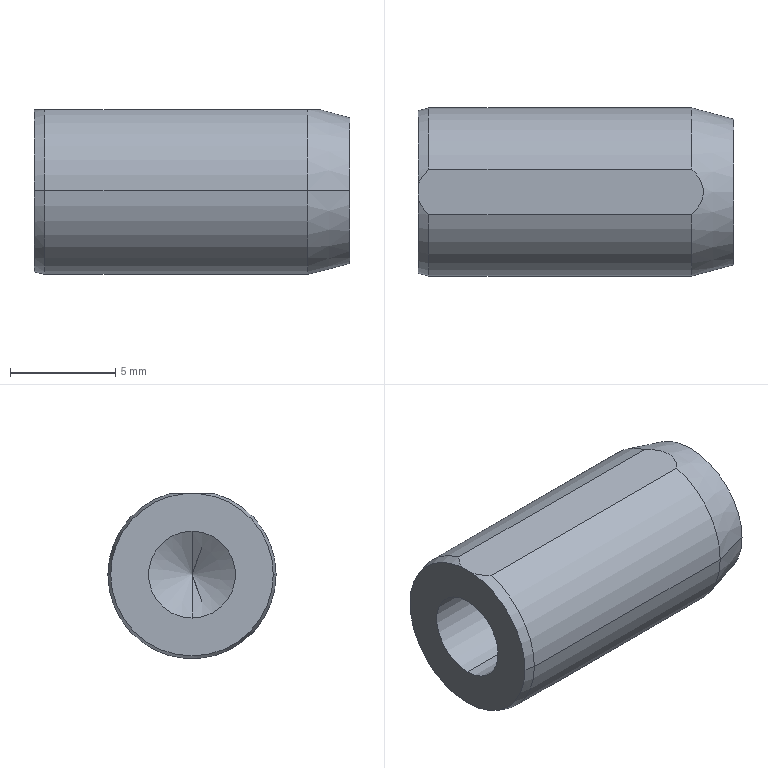Part | STEP file | MSTMS8-15-4 | 1 solid | 15 faces | box 15 x 8 x 7.85 mm | volume 624.527 mm3 | cone 7 | cylinder 5 | plane 3 | commonest cylinder face diameters 8 x3 4.134 x2
STEP:
#1=CARTESIAN_POINT('',(0.,0.,0.));
#2=DIRECTION('',(0.,0.,1.));
#3=DIRECTION('',(1.,0.,0.));
#4=AXIS2_PLACEMENT_3D('',#1,#2,#3);
#5=CARTESIAN_POINT('',(-7.,0.,2.067));
#6=VERTEX_POINT('',#5);
#7=CARTESIAN_POINT('',(-15.,0.,2.067));
#8=VERTEX_POINT('',#7);
#9=CARTESIAN_POINT('',(-15.,0.,2.067));
#10=DIRECTION('',(-1.,0.,0.));
#11=VECTOR('',#10,1.);
#12=LINE('',#9,#11);
#13=CARTESIAN_POINT('',(-15.,0.,0.));
#14=DIRECTION('',(-1.,0.,0.));
#15=DIRECTION('',(0.,0.,1.));
#16=AXIS2_PLACEMENT_3D('',#13,#14,#15);
#17=CYLINDRICAL_SURFACE('',#16,2.067);
#18=CARTESIAN_POINT('',(6.283,0.));
#19=DIRECTION('',(0.,1.));
#20=VECTOR('',#19,1.);
#21=LINE('',#18,#20);
#22=(GEOMETRIC_REPRESENTATION_CONTEXT(2)PARAMETRIC_REPRESENTATION_CONTEXT()REPRESENTATION_CONTEXT('',''));
#23=DEFINITIONAL_REPRESENTATION('',(#21),#22);
#24=PCURVE('',#17,#23);
#25=CARTESIAN_POINT('',(-15.,0.,0.));
#26=DIRECTION('',(-1.,0.,0.));
#27=DIRECTION('',(0.,0.,1.));
#28=AXIS2_PLACEMENT_3D('',#25,#26,#27);
#29=CYLINDRICAL_SURFACE('',#28,2.067);
#30=CARTESIAN_POINT('',(0.,0.));
#31=DIRECTION('',(0.,1.));
#32=VECTOR('',#31,1.);
#33=LINE('',#30,#32);
#34=(GEOMETRIC_REPRESENTATION_CONTEXT(2)PARAMETRIC_REPRESENTATION_CONTEXT()REPRESENTATION_CONTEXT('',''));
#35=DEFINITIONAL_REPRESENTATION('',(#33),#34);
#36=PCURVE('',#29,#35);
#37=SURFACE_CURVE('',#12,(#24,#36),.PCURVE_S1.);
#38=EDGE_CURVE('',#6,#8,#37,.T.);
#39=ORIENTED_EDGE('',*,*,#38,.T.);
#40=CARTESIAN_POINT('',(-15.,0.,-2.067));
#41=VERTEX_POINT('',#40);
#42=CARTESIAN_POINT('',(-15.,0.,0.));
#43=DIRECTION('',(-1.,0.,0.));
#44=DIRECTION('',(0.,0.,1.));
#45=AXIS2_PLACEMENT_3D('',#42,#43,#44);
#46=CIRCLE('',#45,2.067);
#47=CARTESIAN_POINT('',(0.,0.));
#48=DIRECTION('',(1.,0.));
#49=VECTOR('',#48,1.);
#50=LINE('',#47,#49);
#51=(GEOMETRIC_REPRESENTATION_CONTEXT(2)PARAMETRIC_REPRESENTATION_CONTEXT()REPRESENTATION_CONTEXT('',''));
#52=DEFINITIONAL_REPRESENTATION('',(#50),#51);
#53=PCURVE('',#17,#52);
#54=CARTESIAN_POINT('',(-15.,0.,0.));
#55=DIRECTION('',(-1.,0.,0.));
#56=DIRECTION('',(0.,-1.,0.));
#57=AXIS2_PLACEMENT_3D('',#54,#55,#56);
#58=PLANE('',#57);
#59=CARTESIAN_POINT('',(0.,0.));
#60=DIRECTION('',(0.,1.));
#61=AXIS2_PLACEMENT_2D('',#59,#60);
#62=CIRCLE('',#61,2.067);
#63=(GEOMETRIC_REPRESENTATION_CONTEXT(2)PARAMETRIC_REPRESENTATION_CONTEXT()REPRESENTATION_CONTEXT('',''));
#64=DEFINITIONAL_REPRESENTATION('',(#62),#63);
#65=PCURVE('',#58,#64);
#66=SURFACE_CURVE('',#46,(#53,#65),.PCURVE_S1.);
#67=EDGE_CURVE('',#41,#8,#66,.T.);
#68=ORIENTED_EDGE('',*,*,#67,.F.);
#69=CARTESIAN_POINT('',(-7.,0.,-2.067));
#70=VERTEX_POINT('',#69);
#71=CARTESIAN_POINT('',(-15.,0.,-2.067));
#72=DIRECTION('',(-1.,0.,0.));
#73=VECTOR('',#72,1.);
#74=LINE('',#71,#73);
#75=CARTESIAN_POINT('',(3.142,0.));
#76=DIRECTION('',(0.,1.));
#77=VECTOR('',#76,1.);
#78=LINE('',#75,#77);
#79=(GEOMETRIC_REPRESENTATION_CONTEXT(2)PARAMETRIC_REPRESENTATION_CONTEXT()REPRESENTATION_CONTEXT('',''));
#80=DEFINITIONAL_REPRESENTATION('',(#78),#79);
#81=PCURVE('',#17,#80);
#82=CARTESIAN_POINT('',(3.142,0.));
#83=DIRECTION('',(0.,1.));
#84=VECTOR('',#83,1.);
#85=LINE('',#82,#84);
#86=(GEOMETRIC_REPRESENTATION_CONTEXT(2)PARAMETRIC_REPRESENTATION_CONTEXT()REPRESENTATION_CONTEXT('',''));
#87=DEFINITIONAL_REPRESENTATION('',(#85),#86);
#88=PCURVE('',#29,#87);
#89=SURFACE_CURVE('',#74,(#81,#88),.PCURVE_S1.);
#90=EDGE_CURVE('',#70,#41,#89,.T.);
#91=ORIENTED_EDGE('',*,*,#90,.F.);
#92=CARTESIAN_POINT('',(-7.,0.,0.));
#93=DIRECTION('',(-1.,0.,0.));
#94=DIRECTION('',(0.,0.,1.));
#95=AXIS2_PLACEMENT_3D('',#92,#93,#94);
#96=CIRCLE('',#95,2.067);
#97=CARTESIAN_POINT('',(0.,-8.));
#98=DIRECTION('',(1.,0.));
#99=VECTOR('',#98,1.);
#100=LINE('',#97,#99);
#101=(GEOMETRIC_REPRESENTATION_CONTEXT(2)PARAMETRIC_REPRESENTATION_CONTEXT()REPRESENTATION_CONTEXT('',''));
#102=DEFINITIONAL_REPRESENTATION('',(#100),#101);
#103=PCURVE('',#17,#102);
#104=CARTESIAN_POINT('',(-7.,0.,0.));
#105=DIRECTION('',(-1.,0.,0.));
#106=DIRECTION('',(0.,0.,1.));
#107=AXIS2_PLACEMENT_3D('',#104,#105,#106);
#108=CONICAL_SURFACE('',#107,2.067,1.03);
#109=CARTESIAN_POINT('',(0.,0.));
#110=DIRECTION('',(1.,0.));
#111=VECTOR('',#110,1.);
#112=LINE('',#109,#111);
#113=(GEOMETRIC_REPRESENTATION_CONTEXT(2)PARAMETRIC_REPRESENTATION_CONTEXT()REPRESENTATION_CONTEXT('',''));
#114=DEFINITIONAL_REPRESENTATION('',(#112),#113);
#115=PCURVE('',#108,#114);
#116=SURFACE_CURVE('',#96,(#103,#115),.PCURVE_S1.);
#117=EDGE_CURVE('',#70,#6,#116,.T.);
#118=ORIENTED_EDGE('',*,*,#117,.T.);
#119=EDGE_LOOP('',(#39,#68,#91,#118));
#120=FACE_BOUND('',#119,.F.);
#121=ADVANCED_FACE('',(#120),#17,.F.);
#122=ORIENTED_EDGE('',*,*,#117,.F.);
#123=CARTESIAN_POINT('',(-5.758,0.,0.));
#124=VERTEX_POINT('',#123);
#125=CARTESIAN_POINT('',(-7.,0.,-2.067));
#126=DIRECTION('',(-0.515,0.,-0.8572));
#127=VECTOR('',#126,1.);
#128=LINE('',#125,#127);
#129=CARTESIAN_POINT('',(3.142,0.));
#130=DIRECTION('',(0.,1.));
#131=VECTOR('',#130,1.);
#132=LINE('',#129,#131);
#133=(GEOMETRIC_REPRESENTATION_CONTEXT(2)PARAMETRIC_REPRESENTATION_CONTEXT()REPRESENTATION_CONTEXT('',''));
#134=DEFINITIONAL_REPRESENTATION('',(#132),#133);
#135=PCURVE('',#108,#134);
#136=CARTESIAN_POINT('',(-7.,0.,0.));
#137=DIRECTION('',(-1.,0.,0.));
#138=DIRECTION('',(0.,0.,1.));
#139=AXIS2_PLACEMENT_3D('',#136,#137,#138);
#140=CONICAL_SURFACE('',#139,2.067,1.03);
#141=CARTESIAN_POINT('',(3.142,0.));
#142=DIRECTION('',(0.,1.));
#143=VECTOR('',#142,1.);
#144=LINE('',#141,#143);
#145=(GEOMETRIC_REPRESENTATION_CONTEXT(2)PARAMETRIC_REPRESENTATION_CONTEXT()REPRESENTATION_CONTEXT('',''));
#146=DEFINITIONAL_REPRESENTATION('',(#144),#145);
#147=PCURVE('',#140,#146);
#148=SURFACE_CURVE('',#128,(#135,#147),.PCURVE_S1.);
#149=EDGE_CURVE('',#124,#70,#148,.T.);
#150=ORIENTED_EDGE('',*,*,#149,.F.);
#151=CARTESIAN_POINT('',(-7.,0.,2.067));
#152=DIRECTION('',(-0.515,0.,0.8572));
#153=VECTOR('',#152,1.);
#154=LINE('',#151,#153);
#155=CARTESIAN_POINT('',(6.283,0.));
#156=DIRECTION('',(0.,1.));
#157=VECTOR('',#156,1.);
#158=LINE('',#155,#157);
#159=(GEOMETRIC_REPRESENTATION_CONTEXT(2)PARAMETRIC_REPRESENTATION_CONTEXT()REPRESENTATION_CONTEXT('',''));
#160=DEFINITIONAL_REPRESENTATION('',(#158),#159);
#161=PCURVE('',#108,#160);
#162=CARTESIAN_POINT('',(0.,0.));
#163=DIRECTION('',(0.,1.));
#164=VECTOR('',#163,1.);
#165=LINE('',#162,#164);
#166=(GEOMETRIC_REPRESENTATION_CONTEXT(2)PARAMETRIC_REPRESENTATION_CONTEXT()REPRESENTATION_CONTEXT('',''));
#167=DEFINITIONAL_REPRESENTATION('',(#165),#166);
#168=PCURVE('',#140,#167);
#169=SURFACE_CURVE('',#154,(#161,#168),.PCURVE_S1.);
#170=EDGE_CURVE('',#124,#6,#169,.T.);
#171=ORIENTED_EDGE('',*,*,#170,.T.);
#172=EDGE_LOOP('',(#122,#150,#171));
#173=FACE_BOUND('',#172,.F.);
#174=ADVANCED_FACE('',(#173),#108,.F.);
#175=CARTESIAN_POINT('',(0.,3.464,0.));
#176=VERTEX_POINT('',#175);
#177=CARTESIAN_POINT('',(0.,-3.464,0.));
#178=VERTEX_POINT('',#177);
#179=CARTESIAN_POINT('',(0.,0.,0.));
#180=DIRECTION('',(1.,0.,0.));
#181=DIRECTION('',(0.,1.,0.));
#182=AXIS2_PLACEMENT_3D('',#179,#180,#181);
#183=CIRCLE('',#182,3.464);
#184=CARTESIAN_POINT('',(0.,0.,0.));
#185=DIRECTION('',(-1.,0.,0.));
#186=DIRECTION('',(0.,-1.,0.));
#187=AXIS2_PLACEMENT_3D('',#184,#185,#186);
#188=CONICAL_SURFACE('',#187,3.464,0.2618);
#189=CARTESIAN_POINT('',(3.142,0.));
#190=DIRECTION('',(-1.,0.));
#191=VECTOR('',#190,1.);
#192=LINE('',#189,#191);
#193=(GEOMETRIC_REPRESENTATION_CONTEXT(2)PARAMETRIC_REPRESENTATION_CONTEXT()REPRESENTATION_CONTEXT('',''));
#194=DEFINITIONAL_REPRESENTATION('',(#192),#193);
#195=PCURVE('',#188,#194);
#196=CARTESIAN_POINT('',(0.,0.,0.));
#197=DIRECTION('',(1.,0.,0.));
#198=DIRECTION('',(0.,1.,0.));
#199=AXIS2_PLACEMENT_3D('',#196,#197,#198);
#200=PLANE('',#199);
#201=CARTESIAN_POINT('',(0.,0.));
#202=DIRECTION('',(1.,0.));
#203=AXIS2_PLACEMENT_2D('',#201,#202);
#204=CIRCLE('',#203,3.464);
#205=(GEOMETRIC_REPRESENTATION_CONTEXT(2)PARAMETRIC_REPRESENTATION_CONTEXT()REPRESENTATION_CONTEXT('',''));
#206=DEFINITIONAL_REPRESENTATION('',(#204),#205);
#207=PCURVE('',#200,#206);
#208=SURFACE_CURVE('',#183,(#195,#207),.PCURVE_S1.);
#209=EDGE_CURVE('',#176,#178,#208,.T.);
#210=ORIENTED_EDGE('',*,*,#209,.F.);
#211=CARTESIAN_POINT('',(-2.,4.,0.));
#212=VERTEX_POINT('',#211);
#213=CARTESIAN_POINT('',(0.,3.464,0.));
#214=DIRECTION('',(-0.9659,0.2588,0.));
#215=VECTOR('',#214,1.);
#216=LINE('',#213,#215);
#217=CARTESIAN_POINT('',(3.142,0.));
#218=DIRECTION('',(0.,1.));
#219=VECTOR('',#218,1.);
#220=LINE('',#217,#219);
#221=(GEOMETRIC_REPRESENTATION_CONTEXT(2)PARAMETRIC_REPRESENTATION_CONTEXT()REPRESENTATION_CONTEXT('',''));
#222=DEFINITIONAL_REPRESENTATION('',(#220),#221);
#223=PCURVE('',#188,#222);
#224=CARTESIAN_POINT('',(0.,0.,0.));
#225=DIRECTION('',(-1.,0.,0.));
#226=DIRECTION('',(0.,-1.,0.));
#227=AXIS2_PLACEMENT_3D('',#224,#225,#226);
#228=CONICAL_SURFACE('',#227,3.464,0.2618);
#229=CARTESIAN_POINT('',(3.142,0.));
#230=DIRECTION('',(0.,1.));
#231=VECTOR('',#230,1.);
#232=LINE('',#229,#231);
#233=(GEOMETRIC_REPRESENTATION_CONTEXT(2)PARAMETRIC_REPRESENTATION_CONTEXT()REPRESENTATION_CONTEXT('',''));
#234=DEFINITIONAL_REPRESENTATION('',(#232),#233);
#235=PCURVE('',#228,#234);
#236=SURFACE_CURVE('',#216,(#223,#235),.PCURVE_S1.);
#237=EDGE_CURVE('',#176,#212,#236,.T.);
#238=ORIENTED_EDGE('',*,*,#237,.T.);
#239=CARTESIAN_POINT('',(-2.,1.085,3.85));
#240=VERTEX_POINT('',#239);
#241=CARTESIAN_POINT('',(-2.,0.,0.));
#242=DIRECTION('',(1.,0.,0.));
#243=DIRECTION('',(0.,1.,0.));
#244=AXIS2_PLACEMENT_3D('',#241,#242,#243);
#245=CIRCLE('',#244,4.);
#246=CARTESIAN_POINT('',(3.142,2.));
#247=DIRECTION('',(-1.,0.));
#248=VECTOR('',#247,1.);
#249=LINE('',#246,#248);
#250=(GEOMETRIC_REPRESENTATION_CONTEXT(2)PARAMETRIC_REPRESENTATION_CONTEXT()REPRESENTATION_CONTEXT('',''));
#251=DEFINITIONAL_REPRESENTATION('',(#249),#250);
#252=PCURVE('',#188,#251);
#253=CARTESIAN_POINT('',(0.,0.,0.));
#254=DIRECTION('',(1.,0.,0.));
#255=DIRECTION('',(0.,1.,0.));
#256=AXIS2_PLACEMENT_3D('',#253,#254,#255);
#257=CYLINDRICAL_SURFACE('',#256,4.);
#258=CARTESIAN_POINT('',(0.,-2.));
#259=DIRECTION('',(1.,0.));
#260=VECTOR('',#259,1.);
#261=LINE('',#258,#260);
#262=(GEOMETRIC_REPRESENTATION_CONTEXT(2)PARAMETRIC_REPRESENTATION_CONTEXT()REPRESENTATION_CONTEXT('',''));
#263=DEFINITIONAL_REPRESENTATION('',(#261),#262);
#264=PCURVE('',#257,#263);
#265=SURFACE_CURVE('',#245,(#252,#264),.PCURVE_S1.);
#266=EDGE_CURVE('',#212,#240,#265,.T.);
#267=ORIENTED_EDGE('',*,*,#266,.T.);
#268=CARTESIAN_POINT('',(-2.,-1.085,3.85));
#269=VERTEX_POINT('',#268);
#270=CARTESIAN_POINT('',(-2.,-1.085,3.85));
#271=CARTESIAN_POINT('',(-1.853,-0.9403,3.85));
#272=CARTESIAN_POINT('',(-1.716,-0.7784,3.85));
#273=CARTESIAN_POINT('',(-1.508,-0.4159,3.85));
#274=CARTESIAN_POINT('',(-1.44,-0.2099,3.85));
#275=CARTESIAN_POINT('',(-1.44,0.2107,3.85));
#276=CARTESIAN_POINT('',(-1.508,0.4155,3.85));
#277=CARTESIAN_POINT('',(-1.663,0.687,3.85));
#278=CARTESIAN_POINT('',(-1.724,0.7735,3.85));
#279=CARTESIAN_POINT('',(-1.856,0.9358,3.85));
#280=CARTESIAN_POINT('',(-1.926,1.012,3.85));
#281=CARTESIAN_POINT('',(-2.,1.085,3.85));
#282=B_SPLINE_CURVE_WITH_KNOTS('',3,(#270,#271,#272,#273,#274,#275,#276,#277,#278,#279,#280,#281),.UNSPECIFIED.,.F.,.F.,(4,2,2,2,2,4),(0.001238,0.001854,0.00247,0.003086,0.003394,0.003702),.UNSPECIFIED.);
#283=CARTESIAN_POINT('',(1.296,2.));
#284=CARTESIAN_POINT('',(1.302,1.973));
#285=CARTESIAN_POINT('',(1.315,1.921));
#286=CARTESIAN_POINT('',(1.336,1.844));
#287=CARTESIAN_POINT('',(1.358,1.771));
#288=CARTESIAN_POINT('',(1.38,1.703));
#289=CARTESIAN_POINT('',(1.404,1.64));
#290=CARTESIAN_POINT('',(1.429,1.583));
#291=CARTESIAN_POINT('',(1.456,1.534));
#292=CARTESIAN_POINT('',(1.483,1.494));
#293=CARTESIAN_POINT('',(1.512,1.464));
#294=CARTESIAN_POINT('',(1.541,1.445));
#295=CARTESIAN_POINT('',(1.571,1.438));
#296=CARTESIAN_POINT('',(1.601,1.445));
#297=CARTESIAN_POINT('',(1.63,1.464));
#298=CARTESIAN_POINT('',(1.658,1.494));
#299=CARTESIAN_POINT('',(1.686,1.534));
#300=CARTESIAN_POINT('',(1.712,1.583));
#301=CARTESIAN_POINT('',(1.737,1.64));
#302=CARTESIAN_POINT('',(1.761,1.703));
#303=CARTESIAN_POINT('',(1.784,1.772));
#304=CARTESIAN_POINT('',(1.806,1.844));
#305=CARTESIAN_POINT('',(1.826,1.92));
#306=CARTESIAN_POINT('',(1.839,1.973));
#307=CARTESIAN_POINT('',(1.846,2.));
#308=B_SPLINE_CURVE_WITH_KNOTS('',3,(#283,#284,#285,#286,#287,#288,#289,#290,#291,#292,#293,#294,#295,#296,#297,#298,#299,#300,#301,#302,#303,#304,#305,#306,#307),.UNSPECIFIED.,.F.,.F.,(4,1,1,1,1,1,1,1,1,1,1,1,1,1,1,1,1,1,1,1,1,1,4),(0.001238,0.00135,0.001462,0.001574,0.001686,0.001798,0.00191,0.002022,0.002134,0.002246,0.002358,0.00247,0.002582,0.002694,0.002806,0.002918,0.00303,0.003142,0.003254,0.003366,0.003478,0.00359,0.003702),.QUASI_UNIFORM_KNOTS.);
#309=(GEOMETRIC_REPRESENTATION_CONTEXT(2)PARAMETRIC_REPRESENTATION_CONTEXT()REPRESENTATION_CONTEXT('',''));
#310=DEFINITIONAL_REPRESENTATION('',(#308),#309);
#311=PCURVE('',#188,#310);
#312=CARTESIAN_POINT('',(-15.,1.085,3.85));
#313=DIRECTION('',(0.,0.,-1.));
#314=DIRECTION('',(-1.,0.,0.));
#315=AXIS2_PLACEMENT_3D('',#312,#313,#314);
#316=PLANE('',#315);
#317=CARTESIAN_POINT('',(-13.,-2.17));
#318=CARTESIAN_POINT('',(-13.147,-2.025));
#319=CARTESIAN_POINT('',(-13.284,-1.864));
#320=CARTESIAN_POINT('',(-13.492,-1.501));
#321=CARTESIAN_POINT('',(-13.56,-1.295));
#322=CARTESIAN_POINT('',(-13.56,-0.8744));
#323=CARTESIAN_POINT('',(-13.492,-0.6696));
#324=CARTESIAN_POINT('',(-13.337,-0.3981));
#325=CARTESIAN_POINT('',(-13.276,-0.3116));
#326=CARTESIAN_POINT('',(-13.144,-0.1493));
#327=CARTESIAN_POINT('',(-13.074,-0.07297));
#328=CARTESIAN_POINT('',(-13.,0.));
#329=B_SPLINE_CURVE_WITH_KNOTS('',3,(#317,#318,#319,#320,#321,#322,#323,#324,#325,#326,#327,#328),.UNSPECIFIED.,.F.,.F.,(4,2,2,2,2,4),(0.001238,0.001854,0.00247,0.003086,0.003394,0.003702),.UNSPECIFIED.);
#330=(GEOMETRIC_REPRESENTATION_CONTEXT(2)PARAMETRIC_REPRESENTATION_CONTEXT()REPRESENTATION_CONTEXT('',''));
#331=DEFINITIONAL_REPRESENTATION('',(#329),#330);
#332=PCURVE('',#316,#331);
#333=SURFACE_CURVE('',#282,(#311,#332),.PCURVE_S1.);
#334=EDGE_CURVE('',#269,#240,#333,.T.);
#335=ORIENTED_EDGE('',*,*,#334,.F.);
#336=CARTESIAN_POINT('',(-2.,-4.,0.));
#337=VERTEX_POINT('',#336);
#338=CARTESIAN_POINT('',(-2.,0.,0.));
#339=DIRECTION('',(1.,0.,0.));
#340=DIRECTION('',(0.,1.,0.));
#341=AXIS2_PLACEMENT_3D('',#338,#339,#340);
#342=CIRCLE('',#341,4.);
#343=CARTESIAN_POINT('',(3.142,2.));
#344=DIRECTION('',(-1.,0.));
#345=VECTOR('',#344,1.);
#346=LINE('',#343,#345);
#347=(GEOMETRIC_REPRESENTATION_CONTEXT(2)PARAMETRIC_REPRESENTATION_CONTEXT()REPRESENTATION_CONTEXT('',''));
#348=DEFINITIONAL_REPRESENTATION('',(#346),#347);
#349=PCURVE('',#188,#348);
#350=CARTESIAN_POINT('',(0.,0.,0.));
#351=DIRECTION('',(1.,0.,0.));
#352=DIRECTION('',(0.,1.,0.));
#353=AXIS2_PLACEMENT_3D('',#350,#351,#352);
#354=CYLINDRICAL_SURFACE('',#353,4.);
#355=CARTESIAN_POINT('',(0.,-2.));
#356=DIRECTION('',(1.,0.));
#357=VECTOR('',#356,1.);
#358=LINE('',#355,#357);
#359=(GEOMETRIC_REPRESENTATION_CONTEXT(2)PARAMETRIC_REPRESENTATION_CONTEXT()REPRESENTATION_CONTEXT('',''));
#360=DEFINITIONAL_REPRESENTATION('',(#358),#359);
#361=PCURVE('',#354,#360);
#362=SURFACE_CURVE('',#342,(#349,#361),.PCURVE_S1.);
#363=EDGE_CURVE('',#269,#337,#362,.T.);
#364=ORIENTED_EDGE('',*,*,#363,.T.);
#365=CARTESIAN_POINT('',(0.,-3.464,0.));
#366=DIRECTION('',(-0.9659,-0.2588,0.));
#367=VECTOR('',#366,1.);
#368=LINE('',#365,#367);
#369=CARTESIAN_POINT('',(0.,0.));
#370=DIRECTION('',(0.,1.));
#371=VECTOR('',#370,1.);
#372=LINE('',#369,#371);
#373=(GEOMETRIC_REPRESENTATION_CONTEXT(2)PARAMETRIC_REPRESENTATION_CONTEXT()REPRESENTATION_CONTEXT('',''));
#374=DEFINITIONAL_REPRESENTATION('',(#372),#373);
#375=PCURVE('',#188,#374);
#376=CARTESIAN_POINT('',(6.283,0.));
#377=DIRECTION('',(0.,1.));
#378=VECTOR('',#377,1.);
#379=LINE('',#376,#378);
#380=(GEOMETRIC_REPRESENTATION_CONTEXT(2)PARAMETRIC_REPRESENTATION_CONTEXT()REPRESENTATION_CONTEXT('',''));
#381=DEFINITIONAL_REPRESENTATION('',(#379),#380);
#382=PCURVE('',#228,#381);
#383=SURFACE_CURVE('',#368,(#375,#382),.PCURVE_S1.);
#384=EDGE_CURVE('',#178,#337,#383,.T.);
#385=ORIENTED_EDGE('',*,*,#384,.F.);
#386=EDGE_LOOP('',(#210,#238,#267,#335,#364,#385));
#387=FACE_BOUND('',#386,.T.);
#388=ADVANCED_FACE('',(#387),#188,.T.);
#389=CARTESIAN_POINT('',(-14.5,-1.085,3.85));
#390=VERTEX_POINT('',#389);
#391=CARTESIAN_POINT('',(-14.5,-4.,0.));
#392=VERTEX_POINT('',#391);
#393=CARTESIAN_POINT('',(-14.5,0.,0.));
#394=DIRECTION('',(1.,0.,0.));
#395=DIRECTION('',(0.,1.,0.));
#396=AXIS2_PLACEMENT_3D('',#393,#394,#395);
#397=CIRCLE('',#396,4.);
#398=CARTESIAN_POINT('',(0.,-14.5));
#399=DIRECTION('',(1.,0.));
#400=VECTOR('',#399,1.);
#401=LINE('',#398,#400);
#402=(GEOMETRIC_REPRESENTATION_CONTEXT(2)PARAMETRIC_REPRESENTATION_CONTEXT()REPRESENTATION_CONTEXT('',''));
#403=DEFINITIONAL_REPRESENTATION('',(#401),#402);
#404=PCURVE('',#354,#403);
#405=CARTESIAN_POINT('',(-14.5,0.,0.));
#406=DIRECTION('',(1.,0.,0.));
#407=DIRECTION('',(0.,1.,0.));
#408=AXIS2_PLACEMENT_3D('',#405,#406,#407);
#409=CONICAL_SURFACE('',#408,4.,0.2618);
#410=CARTESIAN_POINT('',(0.,0.));
#411=DIRECTION('',(1.,0.));
#412=VECTOR('',#411,1.);
#413=LINE('',#410,#412);
#414=(GEOMETRIC_REPRESENTATION_CONTEXT(2)PARAMETRIC_REPRESENTATION_CONTEXT()REPRESENTATION_CONTEXT('',''));
#415=DEFINITIONAL_REPRESENTATION('',(#413),#414);
#416=PCURVE('',#409,#415);
#417=SURFACE_CURVE('',#397,(#404,#416),.PCURVE_S1.);
#418=EDGE_CURVE('',#390,#392,#417,.T.);
#419=ORIENTED_EDGE('',*,*,#418,.T.);
#420=CARTESIAN_POINT('',(0.,-4.,0.));
#421=DIRECTION('',(1.,0.,0.));
#422=VECTOR('',#421,1.);
#423=LINE('',#420,#422);
#424=CARTESIAN_POINT('',(3.142,0.));
#425=DIRECTION('',(0.,1.));
#426=VECTOR('',#425,1.);
#427=LINE('',#424,#426);
#428=(GEOMETRIC_REPRESENTATION_CONTEXT(2)PARAMETRIC_REPRESENTATION_CONTEXT()REPRESENTATION_CONTEXT('',''));
#429=DEFINITIONAL_REPRESENTATION('',(#427),#428);
#430=PCURVE('',#354,#429);
#431=CARTESIAN_POINT('',(0.,0.,0.));
#432=DIRECTION('',(1.,0.,0.));
#433=DIRECTION('',(0.,1.,0.));
#434=AXIS2_PLACEMENT_3D('',#431,#432,#433);
#435=CYLINDRICAL_SURFACE('',#434,4.);
#436=CARTESIAN_POINT('',(3.142,0.));
#437=DIRECTION('',(0.,1.));
#438=VECTOR('',#437,1.);
#439=LINE('',#436,#438);
#440=(GEOMETRIC_REPRESENTATION_CONTEXT(2)PARAMETRIC_REPRESENTATION_CONTEXT()REPRESENTATION_CONTEXT('',''));
#441=DEFINITIONAL_REPRESENTATION('',(#439),#440);
#442=PCURVE('',#435,#441);
#443=SURFACE_CURVE('',#423,(#430,#442),.PCURVE_S1.);
#444=EDGE_CURVE('',#392,#337,#443,.T.);
#445=ORIENTED_EDGE('',*,*,#444,.T.);
#446=ORIENTED_EDGE('',*,*,#363,.F.);
#447=CARTESIAN_POINT('',(-15.,-1.085,3.85));
#448=DIRECTION('',(1.,0.,0.));
#449=VECTOR('',#448,1.);
#450=LINE('',#447,#449);
#451=CARTESIAN_POINT('',(1.846,-15.));
#452=DIRECTION('',(0.,1.));
#453=VECTOR('',#452,1.);
#454=LINE('',#451,#453);
#455=(GEOMETRIC_REPRESENTATION_CONTEXT(2)PARAMETRIC_REPRESENTATION_CONTEXT()REPRESENTATION_CONTEXT('',''));
#456=DEFINITIONAL_REPRESENTATION('',(#454),#455);
#457=PCURVE('',#354,#456);
#458=CARTESIAN_POINT('',(0.,-2.17));
#459=DIRECTION('',(-1.,0.));
#460=VECTOR('',#459,1.);
#461=LINE('',#458,#460);
#462=(GEOMETRIC_REPRESENTATION_CONTEXT(2)PARAMETRIC_REPRESENTATION_CONTEXT()REPRESENTATION_CONTEXT('',''));
#463=DEFINITIONAL_REPRESENTATION('',(#461),#462);
#464=PCURVE('',#316,#463);
#465=SURFACE_CURVE('',#450,(#457,#464),.PCURVE_S1.);
#466=EDGE_CURVE('',#390,#269,#465,.T.);
#467=ORIENTED_EDGE('',*,*,#466,.F.);
#468=EDGE_LOOP('',(#419,#445,#446,#467));
#469=FACE_BOUND('',#468,.T.);
#470=ADVANCED_FACE('',(#469),#354,.T.);
#471=ORIENTED_EDGE('',*,*,#444,.F.);
#472=CARTESIAN_POINT('',(-14.5,4.,0.));
#473=VERTEX_POINT('',#472);
#474=CARTESIAN_POINT('',(-14.5,0.,0.));
#475=DIRECTION('',(1.,0.,0.));
#476=DIRECTION('',(0.,1.,0.));
#477=AXIS2_PLACEMENT_3D('',#474,#475,#476);
#478=CIRCLE('',#477,4.);
#479=CARTESIAN_POINT('',(0.,-14.5));
#480=DIRECTION('',(1.,0.));
#481=VECTOR('',#480,1.);
#482=LINE('',#479,#481);
#483=(GEOMETRIC_REPRESENTATION_CONTEXT(2)PARAMETRIC_REPRESENTATION_CONTEXT()REPRESENTATION_CONTEXT('',''));
#484=DEFINITIONAL_REPRESENTATION('',(#482),#483);
#485=PCURVE('',#435,#484);
#486=CARTESIAN_POINT('',(-14.5,0.,0.));
#487=DIRECTION('',(1.,0.,0.));
#488=DIRECTION('',(0.,1.,0.));
#489=AXIS2_PLACEMENT_3D('',#486,#487,#488);
#490=CONICAL_SURFACE('',#489,4.,0.2618);
#491=CARTESIAN_POINT('',(0.,0.));
#492=DIRECTION('',(1.,0.));
#493=VECTOR('',#492,1.);
#494=LINE('',#491,#493);
#495=(GEOMETRIC_REPRESENTATION_CONTEXT(2)PARAMETRIC_REPRESENTATION_CONTEXT()REPRESENTATION_CONTEXT('',''));
#496=DEFINITIONAL_REPRESENTATION('',(#494),#495);
#497=PCURVE('',#490,#496);
#498=SURFACE_CURVE('',#478,(#485,#497),.PCURVE_S1.);
#499=EDGE_CURVE('',#392,#473,#498,.T.);
#500=ORIENTED_EDGE('',*,*,#499,.T.);
#501=CARTESIAN_POINT('',(0.,4.,0.));
#502=DIRECTION('',(1.,0.,0.));
#503=VECTOR('',#502,1.);
#504=LINE('',#501,#503);
#505=CARTESIAN_POINT('',(6.283,0.));
#506=DIRECTION('',(0.,1.));
#507=VECTOR('',#506,1.);
#508=LINE('',#505,#507);
#509=(GEOMETRIC_REPRESENTATION_CONTEXT(2)PARAMETRIC_REPRESENTATION_CONTEXT()REPRESENTATION_CONTEXT('',''));
#510=DEFINITIONAL_REPRESENTATION('',(#508),#509);
#511=PCURVE('',#435,#510);
#512=CARTESIAN_POINT('',(0.,0.));
#513=DIRECTION('',(0.,1.));
#514=VECTOR('',#513,1.);
#515=LINE('',#512,#514);
#516=(GEOMETRIC_REPRESENTATION_CONTEXT(2)PARAMETRIC_REPRESENTATION_CONTEXT()REPRESENTATION_CONTEXT('',''));
#517=DEFINITIONAL_REPRESENTATION('',(#515),#516);
#518=PCURVE('',#257,#517);
#519=SURFACE_CURVE('',#504,(#511,#518),.PCURVE_S1.);
#520=EDGE_CURVE('',#473,#212,#519,.T.);
#521=ORIENTED_EDGE('',*,*,#520,.T.);
#522=CARTESIAN_POINT('',(-2.,0.,0.));
#523=DIRECTION('',(1.,0.,0.));
#524=DIRECTION('',(0.,1.,0.));
#525=AXIS2_PLACEMENT_3D('',#522,#523,#524);
#526=CIRCLE('',#525,4.);
#527=CARTESIAN_POINT('',(0.,-2.));
#528=DIRECTION('',(1.,0.));
#529=VECTOR('',#528,1.);
#530=LINE('',#527,#529);
#531=(GEOMETRIC_REPRESENTATION_CONTEXT(2)PARAMETRIC_REPRESENTATION_CONTEXT()REPRESENTATION_CONTEXT('',''));
#532=DEFINITIONAL_REPRESENTATION('',(#530),#531);
#533=PCURVE('',#435,#532);
#534=CARTESIAN_POINT('',(9.425,2.));
#535=DIRECTION('',(-1.,0.));
#536=VECTOR('',#535,1.);
#537=LINE('',#534,#536);
#538=(GEOMETRIC_REPRESENTATION_CONTEXT(2)PARAMETRIC_REPRESENTATION_CONTEXT()REPRESENTATION_CONTEXT('',''));
#539=DEFINITIONAL_REPRESENTATION('',(#537),#538);
#540=PCURVE('',#228,#539);
#541=SURFACE_CURVE('',#526,(#533,#540),.PCURVE_S1.);
#542=EDGE_CURVE('',#337,#212,#541,.T.);
#543=ORIENTED_EDGE('',*,*,#542,.F.);
#544=EDGE_LOOP('',(#471,#500,#521,#543));
#545=FACE_BOUND('',#544,.T.);
#546=ADVANCED_FACE('',(#545),#435,.T.);
#547=CARTESIAN_POINT('',(-15.,-0.3516,3.85));
#548=VERTEX_POINT('',#547);
#549=CARTESIAN_POINT('',(-15.,-3.866,0.));
#550=VERTEX_POINT('',#549);
#551=CARTESIAN_POINT('',(-15.,0.,0.));
#552=DIRECTION('',(1.,0.,0.));
#553=DIRECTION('',(0.,1.,0.));
#554=AXIS2_PLACEMENT_3D('',#551,#552,#553);
#555=CIRCLE('',#554,3.866);
#556=CARTESIAN_POINT('',(0.,-0.5));
#557=DIRECTION('',(1.,0.));
#558=VECTOR('',#557,1.);
#559=LINE('',#556,#558);
#560=(GEOMETRIC_REPRESENTATION_CONTEXT(2)PARAMETRIC_REPRESENTATION_CONTEXT()REPRESENTATION_CONTEXT('',''));
#561=DEFINITIONAL_REPRESENTATION('',(#559),#560);
#562=PCURVE('',#409,#561);
#563=CARTESIAN_POINT('',(-3.866,0.));
#564=CARTESIAN_POINT('',(-3.866,6.696));
#565=CARTESIAN_POINT('',(1.933,3.348));
#566=CARTESIAN_POINT('',(7.732,0.));
#567=CARTESIAN_POINT('',(1.933,-3.348));
#568=CARTESIAN_POINT('',(-3.866,-6.696));
#569=CARTESIAN_POINT('',(-3.866,0.));
#570=(BOUNDED_CURVE()B_SPLINE_CURVE(2,(#563,#564,#565,#566,#567,#568,#569),.UNSPECIFIED.,.T.,.F.)B_SPLINE_CURVE_WITH_KNOTS((1,2,2,2,2,1),(-2.094,0.,2.094,4.189,6.283,8.378),.UNSPECIFIED.)CURVE()GEOMETRIC_REPRESENTATION_ITEM()RATIONAL_B_SPLINE_CURVE((1.,0.5,1.,0.5,1.,0.5,1.))REPRESENTATION_ITEM(''));
#571=(GEOMETRIC_REPRESENTATION_CONTEXT(2)PARAMETRIC_REPRESENTATION_CONTEXT()REPRESENTATION_CONTEXT('',''));
#572=DEFINITIONAL_REPRESENTATION('',(#570),#571);
#573=PCURVE('',#58,#572);
#574=SURFACE_CURVE('',#555,(#562,#573),.PCURVE_S1.);
#575=EDGE_CURVE('',#548,#550,#574,.T.);
#576=ORIENTED_EDGE('',*,*,#575,.T.);
#577=CARTESIAN_POINT('',(-14.5,-4.,0.));
#578=DIRECTION('',(0.9659,-0.2588,0.));
#579=VECTOR('',#578,1.);
#580=LINE('',#577,#579);
#581=CARTESIAN_POINT('',(3.142,0.));
#582=DIRECTION('',(0.,1.));
#583=VECTOR('',#582,1.);
#584=LINE('',#581,#583);
#585=(GEOMETRIC_REPRESENTATION_CONTEXT(2)PARAMETRIC_REPRESENTATION_CONTEXT()REPRESENTATION_CONTEXT('',''));
#586=DEFINITIONAL_REPRESENTATION('',(#584),#585);
#587=PCURVE('',#409,#586);
#588=CARTESIAN_POINT('',(3.142,0.));
#589=DIRECTION('',(0.,1.));
#590=VECTOR('',#589,1.);
#591=LINE('',#588,#590);
#592=(GEOMETRIC_REPRESENTATION_CONTEXT(2)PARAMETRIC_REPRESENTATION_CONTEXT()REPRESENTATION_CONTEXT('',''));
#593=DEFINITIONAL_REPRESENTATION('',(#591),#592);
#594=PCURVE('',#490,#593);
#595=SURFACE_CURVE('',#580,(#587,#594),.PCURVE_S1.);
#596=EDGE_CURVE('',#550,#392,#595,.T.);
#597=ORIENTED_EDGE('',*,*,#596,.T.);
#598=ORIENTED_EDGE('',*,*,#418,.F.);
#599=CARTESIAN_POINT('',(-15.,-0.3516,3.85));
#600=CARTESIAN_POINT('',(-14.952,-0.4931,3.85));
#601=CARTESIAN_POINT('',(-14.878,-0.6261,3.85));
#602=CARTESIAN_POINT('',(-14.706,-0.8683,3.85));
#603=CARTESIAN_POINT('',(-14.606,-0.98,3.85));
#604=CARTESIAN_POINT('',(-14.5,-1.085,3.85));
#605=B_SPLINE_CURVE_WITH_KNOTS('',3,(#599,#600,#601,#602,#603,#604),.UNSPECIFIED.,.F.,.F.,(4,2,4),(0.003237,0.003679,0.004122),.UNSPECIFIED.);
#606=CARTESIAN_POINT('',(1.662,-0.5));
#607=CARTESIAN_POINT('',(1.665,-0.4956));
#608=CARTESIAN_POINT('',(1.672,-0.4865));
#609=CARTESIAN_POINT('',(1.682,-0.4715));
#610=CARTESIAN_POINT('',(1.691,-0.4553));
#611=CARTESIAN_POINT('',(1.701,-0.4381));
#612=CARTESIAN_POINT('',(1.71,-0.4198));
#613=CARTESIAN_POINT('',(1.719,-0.4005));
#614=CARTESIAN_POINT('',(1.728,-0.3804));
#615=CARTESIAN_POINT('',(1.737,-0.3593));
#616=CARTESIAN_POINT('',(1.746,-0.3375));
#617=CARTESIAN_POINT('',(1.754,-0.315));
#618=CARTESIAN_POINT('',(1.763,-0.2918));
#619=CARTESIAN_POINT('',(1.771,-0.268));
#620=CARTESIAN_POINT('',(1.779,-0.2436));
#621=CARTESIAN_POINT('',(1.787,-0.2185));
#622=CARTESIAN_POINT('',(1.794,-0.1929));
#623=CARTESIAN_POINT('',(1.802,-0.1668));
#624=CARTESIAN_POINT('',(1.81,-0.1402));
#625=CARTESIAN_POINT('',(1.817,-0.113));
#626=CARTESIAN_POINT('',(1.824,-0.08541));
#627=CARTESIAN_POINT('',(1.832,-0.05736));
#628=CARTESIAN_POINT('',(1.839,-0.02891));
#629=CARTESIAN_POINT('',(1.843,-0.009676));
#630=CARTESIAN_POINT('',(1.846,0.));
#631=B_SPLINE_CURVE_WITH_KNOTS('',3,(#606,#607,#608,#609,#610,#611,#612,#613,#614,#615,#616,#617,#618,#619,#620,#621,#622,#623,#624,#625,#626,#627,#628,#629,#630),.UNSPECIFIED.,.F.,.F.,(4,1,1,1,1,1,1,1,1,1,1,1,1,1,1,1,1,1,1,1,1,1,4),(0.003237,0.003277,0.003317,0.003357,0.003398,0.003438,0.003478,0.003518,0.003559,0.003599,0.003639,0.003679,0.00372,0.00376,0.0038,0.00384,0.003881,0.003921,0.003961,0.004001,0.004042,0.004082,0.004122),.QUASI_UNIFORM_KNOTS.);
#632=(GEOMETRIC_REPRESENTATION_CONTEXT(2)PARAMETRIC_REPRESENTATION_CONTEXT()REPRESENTATION_CONTEXT('',''));
#633=DEFINITIONAL_REPRESENTATION('',(#631),#632);
#634=PCURVE('',#409,#633);
#635=CARTESIAN_POINT('',(0.,-1.437));
#636=CARTESIAN_POINT('',(-0.04803,-1.578));
#637=CARTESIAN_POINT('',(-0.1222,-1.711));
#638=CARTESIAN_POINT('',(-0.2944,-1.953));
#639=CARTESIAN_POINT('',(-0.3936,-2.065));
#640=CARTESIAN_POINT('',(-0.5,-2.17));
#641=B_SPLINE_CURVE_WITH_KNOTS('',3,(#635,#636,#637,#638,#639,#640),.UNSPECIFIED.,.F.,.F.,(4,2,4),(0.003237,0.003679,0.004122),.UNSPECIFIED.);
#642=(GEOMETRIC_REPRESENTATION_CONTEXT(2)PARAMETRIC_REPRESENTATION_CONTEXT()REPRESENTATION_CONTEXT('',''));
#643=DEFINITIONAL_REPRESENTATION('',(#641),#642);
#644=PCURVE('',#316,#643);
#645=SURFACE_CURVE('',#605,(#634,#644),.PCURVE_S1.);
#646=EDGE_CURVE('',#548,#390,#645,.T.);
#647=ORIENTED_EDGE('',*,*,#646,.F.);
#648=EDGE_LOOP('',(#576,#597,#598,#647));
#649=FACE_BOUND('',#648,.T.);
#650=ADVANCED_FACE('',(#649),#409,.T.);
#651=ORIENTED_EDGE('',*,*,#596,.F.);
#652=CARTESIAN_POINT('',(-15.,3.866,0.));
#653=VERTEX_POINT('',#652);
#654=CARTESIAN_POINT('',(-15.,0.,0.));
#655=DIRECTION('',(1.,0.,0.));
#656=DIRECTION('',(0.,1.,0.));
#657=AXIS2_PLACEMENT_3D('',#654,#655,#656);
#658=CIRCLE('',#657,3.866);
#659=CARTESIAN_POINT('',(0.,-0.5));
#660=DIRECTION('',(1.,0.));
#661=VECTOR('',#660,1.);
#662=LINE('',#659,#661);
#663=(GEOMETRIC_REPRESENTATION_CONTEXT(2)PARAMETRIC_REPRESENTATION_CONTEXT()REPRESENTATION_CONTEXT('',''));
#664=DEFINITIONAL_REPRESENTATION('',(#662),#663);
#665=PCURVE('',#490,#664);
#666=CARTESIAN_POINT('',(-3.866,0.));
#667=CARTESIAN_POINT('',(-3.866,6.696));
#668=CARTESIAN_POINT('',(1.933,3.348));
#669=CARTESIAN_POINT('',(7.732,0.));
#670=CARTESIAN_POINT('',(1.933,-3.348));
#671=CARTESIAN_POINT('',(-3.866,-6.696));
#672=CARTESIAN_POINT('',(-3.866,0.));
#673=(BOUNDED_CURVE()B_SPLINE_CURVE(2,(#666,#667,#668,#669,#670,#671,#672),.UNSPECIFIED.,.T.,.F.)B_SPLINE_CURVE_WITH_KNOTS((1,2,2,2,2,1),(-2.094,0.,2.094,4.189,6.283,8.378),.UNSPECIFIED.)CURVE()GEOMETRIC_REPRESENTATION_ITEM()RATIONAL_B_SPLINE_CURVE((1.,0.5,1.,0.5,1.,0.5,1.))REPRESENTATION_ITEM(''));
#674=(GEOMETRIC_REPRESENTATION_CONTEXT(2)PARAMETRIC_REPRESENTATION_CONTEXT()REPRESENTATION_CONTEXT('',''));
#675=DEFINITIONAL_REPRESENTATION('',(#673),#674);
#676=PCURVE('',#58,#675);
#677=SURFACE_CURVE('',#658,(#665,#676),.PCURVE_S1.);
#678=EDGE_CURVE('',#550,#653,#677,.T.);
#679=ORIENTED_EDGE('',*,*,#678,.T.);
#680=CARTESIAN_POINT('',(-14.5,4.,0.));
#681=DIRECTION('',(0.9659,0.2588,0.));
#682=VECTOR('',#681,1.);
#683=LINE('',#680,#682);
#684=CARTESIAN_POINT('',(6.283,0.));
#685=DIRECTION('',(0.,1.));
#686=VECTOR('',#685,1.);
#687=LINE('',#684,#686);
#688=(GEOMETRIC_REPRESENTATION_CONTEXT(2)PARAMETRIC_REPRESENTATION_CONTEXT()REPRESENTATION_CONTEXT('',''));
#689=DEFINITIONAL_REPRESENTATION('',(#687),#688);
#690=PCURVE('',#490,#689);
#691=CARTESIAN_POINT('',(-14.5,0.,0.));
#692=DIRECTION('',(1.,0.,0.));
#693=DIRECTION('',(0.,1.,0.));
#694=AXIS2_PLACEMENT_3D('',#691,#692,#693);
#695=CONICAL_SURFACE('',#694,4.,0.2618);
#696=CARTESIAN_POINT('',(0.,0.));
#697=DIRECTION('',(0.,1.));
#698=VECTOR('',#697,1.);
#699=LINE('',#696,#698);
#700=(GEOMETRIC_REPRESENTATION_CONTEXT(2)PARAMETRIC_REPRESENTATION_CONTEXT()REPRESENTATION_CONTEXT('',''));
#701=DEFINITIONAL_REPRESENTATION('',(#699),#700);
#702=PCURVE('',#695,#701);
#703=SURFACE_CURVE('',#683,(#690,#702),.PCURVE_S1.);
#704=EDGE_CURVE('',#653,#473,#703,.T.);
#705=ORIENTED_EDGE('',*,*,#704,.T.);
#706=ORIENTED_EDGE('',*,*,#499,.F.);
#707=EDGE_LOOP('',(#651,#679,#705,#706));
#708=FACE_BOUND('',#707,.T.);
#709=ADVANCED_FACE('',(#708),#490,.T.);
#710=CARTESIAN_POINT('',(-15.,0.,0.));
#711=DIRECTION('',(-1.,0.,0.));
#712=DIRECTION('',(0.,0.,1.));
#713=AXIS2_PLACEMENT_3D('',#710,#711,#712);
#714=CIRCLE('',#713,2.067);
#715=CARTESIAN_POINT('',(0.,0.));
#716=DIRECTION('',(0.,1.));
#717=AXIS2_PLACEMENT_2D('',#715,#716);
#718=CIRCLE('',#717,2.067);
#719=(GEOMETRIC_REPRESENTATION_CONTEXT(2)PARAMETRIC_REPRESENTATION_CONTEXT()REPRESENTATION_CONTEXT('',''));
#720=DEFINITIONAL_REPRESENTATION('',(#718),#719);
#721=PCURVE('',#58,#720);
#722=CARTESIAN_POINT('',(0.,0.));
#723=DIRECTION('',(1.,0.));
#724=VECTOR('',#723,1.);
#725=LINE('',#722,#724);
#726=(GEOMETRIC_REPRESENTATION_CONTEXT(2)PARAMETRIC_REPRESENTATION_CONTEXT()REPRESENTATION_CONTEXT('',''));
#727=DEFINITIONAL_REPRESENTATION('',(#725),#726);
#728=PCURVE('',#29,#727);
#729=SURFACE_CURVE('',#714,(#721,#728),.PCURVE_S1.);
#730=EDGE_CURVE('',#8,#41,#729,.T.);
#731=ORIENTED_EDGE('',*,*,#730,.F.);
#732=ORIENTED_EDGE('',*,*,#67,.F.);
#733=EDGE_LOOP('',(#731,#732));
#734=FACE_BOUND('',#733,.T.);
#735=CARTESIAN_POINT('',(-15.,0.3516,3.85));
#736=VERTEX_POINT('',#735);
#737=CARTESIAN_POINT('',(-15.,1.085,3.85));
#738=DIRECTION('',(0.,1.,0.));
#739=VECTOR('',#738,1.);
#740=LINE('',#737,#739);
#741=CARTESIAN_POINT('',(-1.085,3.85));
#742=DIRECTION('',(-1.,0.));
#743=VECTOR('',#742,1.);
#744=LINE('',#741,#743);
#745=(GEOMETRIC_REPRESENTATION_CONTEXT(2)PARAMETRIC_REPRESENTATION_CONTEXT()REPRESENTATION_CONTEXT('',''));
#746=DEFINITIONAL_REPRESENTATION('',(#744),#745);
#747=PCURVE('',#58,#746);
#748=CARTESIAN_POINT('',(0.,0.));
#749=DIRECTION('',(0.,1.));
#750=VECTOR('',#749,1.);
#751=LINE('',#748,#750);
#752=(GEOMETRIC_REPRESENTATION_CONTEXT(2)PARAMETRIC_REPRESENTATION_CONTEXT()REPRESENTATION_CONTEXT('',''));
#753=DEFINITIONAL_REPRESENTATION('',(#751),#752);
#754=PCURVE('',#316,#753);
#755=SURFACE_CURVE('',#740,(#747,#754),.PCURVE_S1.);
#756=EDGE_CURVE('',#548,#736,#755,.T.);
#757=ORIENTED_EDGE('',*,*,#756,.T.);
#758=CARTESIAN_POINT('',(-15.,0.,0.));
#759=DIRECTION('',(1.,0.,0.));
#760=DIRECTION('',(0.,1.,0.));
#761=AXIS2_PLACEMENT_3D('',#758,#759,#760);
#762=CIRCLE('',#761,3.866);
#763=CARTESIAN_POINT('',(-3.866,0.));
#764=CARTESIAN_POINT('',(-3.866,6.696));
#765=CARTESIAN_POINT('',(1.933,3.348));
#766=CARTESIAN_POINT('',(7.732,0.));
#767=CARTESIAN_POINT('',(1.933,-3.348));
#768=CARTESIAN_POINT('',(-3.866,-6.696));
#769=CARTESIAN_POINT('',(-3.866,0.));
#770=(BOUNDED_CURVE()B_SPLINE_CURVE(2,(#763,#764,#765,#766,#767,#768,#769),.UNSPECIFIED.,.T.,.F.)B_SPLINE_CURVE_WITH_KNOTS((1,2,2,2,2,1),(-2.094,0.,2.094,4.189,6.283,8.378),.UNSPECIFIED.)CURVE()GEOMETRIC_REPRESENTATION_ITEM()RATIONAL_B_SPLINE_CURVE((1.,0.5,1.,0.5,1.,0.5,1.))REPRESENTATION_ITEM(''));
#771=(GEOMETRIC_REPRESENTATION_CONTEXT(2)PARAMETRIC_REPRESENTATION_CONTEXT()REPRESENTATION_CONTEXT('',''));
#772=DEFINITIONAL_REPRESENTATION('',(#770),#771);
#773=PCURVE('',#58,#772);
#774=CARTESIAN_POINT('',(0.,-0.5));
#775=DIRECTION('',(1.,0.));
#776=VECTOR('',#775,1.);
#777=LINE('',#774,#776);
#778=(GEOMETRIC_REPRESENTATION_CONTEXT(2)PARAMETRIC_REPRESENTATION_CONTEXT()REPRESENTATION_CONTEXT('',''));
#779=DEFINITIONAL_REPRESENTATION('',(#777),#778);
#780=PCURVE('',#695,#779);
#781=SURFACE_CURVE('',#762,(#773,#780),.PCURVE_S1.);
#782=EDGE_CURVE('',#653,#736,#781,.T.);
#783=ORIENTED_EDGE('',*,*,#782,.F.);
#784=ORIENTED_EDGE('',*,*,#678,.F.);
#785=ORIENTED_EDGE('',*,*,#575,.F.);
#786=EDGE_LOOP('',(#757,#783,#784,#785));
#787=FACE_BOUND('',#786,.T.);
#788=ADVANCED_FACE('',(#734,#787),#58,.T.);
#789=ORIENTED_EDGE('',*,*,#704,.F.);
#790=ORIENTED_EDGE('',*,*,#782,.T.);
#791=CARTESIAN_POINT('',(-14.5,1.085,3.85));
#792=VERTEX_POINT('',#791);
#793=CARTESIAN_POINT('',(-14.5,1.085,3.85));
#794=CARTESIAN_POINT('',(-14.606,0.9804,3.85));
#795=CARTESIAN_POINT('',(-14.706,0.868,3.85));
#796=CARTESIAN_POINT('',(-14.878,0.6251,3.85));
#797=CARTESIAN_POINT('',(-14.952,0.4925,3.85));
#798=CARTESIAN_POINT('',(-15.,0.3516,3.85));
#799=B_SPLINE_CURVE_WITH_KNOTS('',3,(#793,#794,#795,#796,#797,#798),.UNSPECIFIED.,.F.,.F.,(4,2,4),(0.001644,0.002086,0.002528),.UNSPECIFIED.);
#800=CARTESIAN_POINT('',(1.296,0.));
#801=CARTESIAN_POINT('',(1.298,-0.009641));
#802=CARTESIAN_POINT('',(1.303,-0.02882));
#803=CARTESIAN_POINT('',(1.31,-0.05725));
#804=CARTESIAN_POINT('',(1.317,-0.0853));
#805=CARTESIAN_POINT('',(1.325,-0.1129));
#806=CARTESIAN_POINT('',(1.332,-0.1401));
#807=CARTESIAN_POINT('',(1.339,-0.1669));
#808=CARTESIAN_POINT('',(1.347,-0.1931));
#809=CARTESIAN_POINT('',(1.355,-0.2188));
#810=CARTESIAN_POINT('',(1.363,-0.2439));
#811=CARTESIAN_POINT('',(1.371,-0.2684));
#812=CARTESIAN_POINT('',(1.379,-0.2923));
#813=CARTESIAN_POINT('',(1.388,-0.3155));
#814=CARTESIAN_POINT('',(1.396,-0.338));
#815=CARTESIAN_POINT('',(1.405,-0.3598));
#816=CARTESIAN_POINT('',(1.414,-0.3808));
#817=CARTESIAN_POINT('',(1.423,-0.4009));
#818=CARTESIAN_POINT('',(1.432,-0.4201));
#819=CARTESIAN_POINT('',(1.441,-0.4384));
#820=CARTESIAN_POINT('',(1.451,-0.4556));
#821=CARTESIAN_POINT('',(1.46,-0.4716));
#822=CARTESIAN_POINT('',(1.47,-0.4865));
#823=CARTESIAN_POINT('',(1.476,-0.4957));
#824=CARTESIAN_POINT('',(1.48,-0.5));
#825=B_SPLINE_CURVE_WITH_KNOTS('',3,(#800,#801,#802,#803,#804,#805,#806,#807,#808,#809,#810,#811,#812,#813,#814,#815,#816,#817,#818,#819,#820,#821,#822,#823,#824),.UNSPECIFIED.,.F.,.F.,(4,1,1,1,1,1,1,1,1,1,1,1,1,1,1,1,1,1,1,1,1,1,4),(0.001644,0.001684,0.001724,0.001764,0.001805,0.001845,0.001885,0.001925,0.001965,0.002006,0.002046,0.002086,0.002126,0.002166,0.002207,0.002247,0.002287,0.002327,0.002368,0.002408,0.002448,0.002488,0.002528),.QUASI_UNIFORM_KNOTS.);
#826=(GEOMETRIC_REPRESENTATION_CONTEXT(2)PARAMETRIC_REPRESENTATION_CONTEXT()REPRESENTATION_CONTEXT('',''));
#827=DEFINITIONAL_REPRESENTATION('',(#825),#826);
#828=PCURVE('',#695,#827);
#829=CARTESIAN_POINT('',(-0.5,0.));
#830=CARTESIAN_POINT('',(-0.3939,-0.1048));
#831=CARTESIAN_POINT('',(-0.2941,-0.2171));
#832=CARTESIAN_POINT('',(-0.1216,-0.46));
#833=CARTESIAN_POINT('',(-0.04781,-0.5926));
#834=CARTESIAN_POINT('',(0.,-0.7335));
#835=B_SPLINE_CURVE_WITH_KNOTS('',3,(#829,#830,#831,#832,#833,#834),.UNSPECIFIED.,.F.,.F.,(4,2,4),(0.001644,0.002086,0.002528),.UNSPECIFIED.);
#836=(GEOMETRIC_REPRESENTATION_CONTEXT(2)PARAMETRIC_REPRESENTATION_CONTEXT()REPRESENTATION_CONTEXT('',''));
#837=DEFINITIONAL_REPRESENTATION('',(#835),#836);
#838=PCURVE('',#316,#837);
#839=SURFACE_CURVE('',#799,(#828,#838),.PCURVE_S1.);
#840=EDGE_CURVE('',#792,#736,#839,.T.);
#841=ORIENTED_EDGE('',*,*,#840,.F.);
#842=CARTESIAN_POINT('',(-14.5,0.,0.));
#843=DIRECTION('',(1.,0.,0.));
#844=DIRECTION('',(0.,1.,0.));
#845=AXIS2_PLACEMENT_3D('',#842,#843,#844);
#846=CIRCLE('',#845,4.);
#847=CARTESIAN_POINT('',(0.,0.));
#848=DIRECTION('',(1.,0.));
#849=VECTOR('',#848,1.);
#850=LINE('',#847,#849);
#851=(GEOMETRIC_REPRESENTATION_CONTEXT(2)PARAMETRIC_REPRESENTATION_CONTEXT()REPRESENTATION_CONTEXT('',''));
#852=DEFINITIONAL_REPRESENTATION('',(#850),#851);
#853=PCURVE('',#695,#852);
#854=CARTESIAN_POINT('',(0.,-14.5));
#855=DIRECTION('',(1.,0.));
#856=VECTOR('',#855,1.);
#857=LINE('',#854,#856);
#858=(GEOMETRIC_REPRESENTATION_CONTEXT(2)PARAMETRIC_REPRESENTATION_CONTEXT()REPRESENTATION_CONTEXT('',''));
#859=DEFINITIONAL_REPRESENTATION('',(#857),#858);
#860=PCURVE('',#257,#859);
#861=SURFACE_CURVE('',#846,(#853,#860),.PCURVE_S1.);
#862=EDGE_CURVE('',#473,#792,#861,.T.);
#863=ORIENTED_EDGE('',*,*,#862,.F.);
#864=EDGE_LOOP('',(#789,#790,#841,#863));
#865=FACE_BOUND('',#864,.T.);
#866=ADVANCED_FACE('',(#865),#695,.T.);
#867=ORIENTED_EDGE('',*,*,#520,.F.);
#868=ORIENTED_EDGE('',*,*,#862,.T.);
#869=CARTESIAN_POINT('',(-15.,1.085,3.85));
#870=DIRECTION('',(1.,0.,0.));
#871=VECTOR('',#870,1.);
#872=LINE('',#869,#871);
#873=CARTESIAN_POINT('',(1.296,-15.));
#874=DIRECTION('',(0.,1.));
#875=VECTOR('',#874,1.);
#876=LINE('',#873,#875);
#877=(GEOMETRIC_REPRESENTATION_CONTEXT(2)PARAMETRIC_REPRESENTATION_CONTEXT()REPRESENTATION_CONTEXT('',''));
#878=DEFINITIONAL_REPRESENTATION('',(#876),#877);
#879=PCURVE('',#257,#878);
#880=CARTESIAN_POINT('',(0.,0.));
#881=DIRECTION('',(-1.,0.));
#882=VECTOR('',#881,1.);
#883=LINE('',#880,#882);
#884=(GEOMETRIC_REPRESENTATION_CONTEXT(2)PARAMETRIC_REPRESENTATION_CONTEXT()REPRESENTATION_CONTEXT('',''));
#885=DEFINITIONAL_REPRESENTATION('',(#883),#884);
#886=PCURVE('',#316,#885);
#887=SURFACE_CURVE('',#872,(#879,#886),.PCURVE_S1.);
#888=EDGE_CURVE('',#792,#240,#887,.T.);
#889=ORIENTED_EDGE('',*,*,#888,.T.);
#890=ORIENTED_EDGE('',*,*,#266,.F.);
#891=EDGE_LOOP('',(#867,#868,#889,#890));
#892=FACE_BOUND('',#891,.T.);
#893=ADVANCED_FACE('',(#892),#257,.T.);
#894=ORIENTED_EDGE('',*,*,#237,.F.);
#895=CARTESIAN_POINT('',(0.,0.,0.));
#896=DIRECTION('',(1.,0.,0.));
#897=DIRECTION('',(0.,1.,0.));
#898=AXIS2_PLACEMENT_3D('',#895,#896,#897);
#899=CIRCLE('',#898,3.464);
#900=CARTESIAN_POINT('',(9.425,0.));
#901=DIRECTION('',(-1.,0.));
#902=VECTOR('',#901,1.);
#903=LINE('',#900,#902);
#904=(GEOMETRIC_REPRESENTATION_CONTEXT(2)PARAMETRIC_REPRESENTATION_CONTEXT()REPRESENTATION_CONTEXT('',''));
#905=DEFINITIONAL_REPRESENTATION('',(#903),#904);
#906=PCURVE('',#228,#905);
#907=CARTESIAN_POINT('',(0.,0.));
#908=DIRECTION('',(1.,0.));
#909=AXIS2_PLACEMENT_2D('',#907,#908);
#910=CIRCLE('',#909,3.464);
#911=(GEOMETRIC_REPRESENTATION_CONTEXT(2)PARAMETRIC_REPRESENTATION_CONTEXT()REPRESENTATION_CONTEXT('',''));
#912=DEFINITIONAL_REPRESENTATION('',(#910),#911);
#913=PCURVE('',#200,#912);
#914=SURFACE_CURVE('',#899,(#906,#913),.PCURVE_S1.);
#915=EDGE_CURVE('',#178,#176,#914,.T.);
#916=ORIENTED_EDGE('',*,*,#915,.F.);
#917=ORIENTED_EDGE('',*,*,#384,.T.);
#918=ORIENTED_EDGE('',*,*,#542,.T.);
#919=EDGE_LOOP('',(#894,#916,#917,#918));
#920=FACE_BOUND('',#919,.T.);
#921=ADVANCED_FACE('',(#920),#228,.T.);
#922=ORIENTED_EDGE('',*,*,#915,.T.);
#923=ORIENTED_EDGE('',*,*,#209,.T.);
#924=EDGE_LOOP('',(#922,#923));
#925=FACE_BOUND('',#924,.T.);
#926=ADVANCED_FACE('',(#925),#200,.T.);
#927=ORIENTED_EDGE('',*,*,#840,.T.);
#928=ORIENTED_EDGE('',*,*,#756,.F.);
#929=ORIENTED_EDGE('',*,*,#646,.T.);
#930=ORIENTED_EDGE('',*,*,#466,.T.);
#931=ORIENTED_EDGE('',*,*,#334,.T.);
#932=ORIENTED_EDGE('',*,*,#888,.F.);
#933=EDGE_LOOP('',(#927,#928,#929,#930,#931,#932));
#934=FACE_BOUND('',#933,.T.);
#935=ADVANCED_FACE('',(#934),#316,.F.);
#936=CARTESIAN_POINT('',(-7.,0.,0.));
#937=DIRECTION('',(-1.,0.,0.));
#938=DIRECTION('',(0.,0.,1.));
#939=AXIS2_PLACEMENT_3D('',#936,#937,#938);
#940=CIRCLE('',#939,2.067);
#941=CARTESIAN_POINT('',(0.,0.));
#942=DIRECTION('',(1.,0.));
#943=VECTOR('',#942,1.);
#944=LINE('',#941,#943);
#945=(GEOMETRIC_REPRESENTATION_CONTEXT(2)PARAMETRIC_REPRESENTATION_CONTEXT()REPRESENTATION_CONTEXT('',''));
#946=DEFINITIONAL_REPRESENTATION('',(#944),#945);
#947=PCURVE('',#140,#946);
#948=CARTESIAN_POINT('',(0.,-8.));
#949=DIRECTION('',(1.,0.));
#950=VECTOR('',#949,1.);
#951=LINE('',#948,#950);
#952=(GEOMETRIC_REPRESENTATION_CONTEXT(2)PARAMETRIC_REPRESENTATION_CONTEXT()REPRESENTATION_CONTEXT('',''));
#953=DEFINITIONAL_REPRESENTATION('',(#951),#952);
#954=PCURVE('',#29,#953);
#955=SURFACE_CURVE('',#940,(#947,#954),.PCURVE_S1.);
#956=EDGE_CURVE('',#6,#70,#955,.T.);
#957=ORIENTED_EDGE('',*,*,#956,.F.);
#958=ORIENTED_EDGE('',*,*,#170,.F.);
#959=ORIENTED_EDGE('',*,*,#149,.T.);
#960=EDGE_LOOP('',(#957,#958,#959));
#961=FACE_BOUND('',#960,.F.);
#962=ADVANCED_FACE('',(#961),#140,.F.);
#963=ORIENTED_EDGE('',*,*,#730,.F.);
#964=ORIENTED_EDGE('',*,*,#38,.F.);
#965=ORIENTED_EDGE('',*,*,#956,.T.);
#966=ORIENTED_EDGE('',*,*,#90,.T.);
#967=EDGE_LOOP('',(#963,#964,#965,#966));
#968=FACE_BOUND('',#967,.F.);
#969=ADVANCED_FACE('',(#968),#29,.F.);
#970=CLOSED_SHELL('',(#121,#174,#388,#470,#546,#650,#709,#788,#866,#893,#921,#926,#935,#962,#969));
#971=MANIFOLD_SOLID_BREP('',#970);
#972=(LENGTH_UNIT()NAMED_UNIT(*)SI_UNIT(.MILLI.,.METRE.));
#973=UNCERTAINTY_MEASURE_WITH_UNIT(LENGTH_MEASURE(0.00002),#972,'','');
#974=(NAMED_UNIT(*)PLANE_ANGLE_UNIT()SI_UNIT($,.RADIAN.));
#975=(NAMED_UNIT(*)SI_UNIT($,.STERADIAN.)SOLID_ANGLE_UNIT());
#976=(GEOMETRIC_REPRESENTATION_CONTEXT(3)GLOBAL_UNCERTAINTY_ASSIGNED_CONTEXT((#973))GLOBAL_UNIT_ASSIGNED_CONTEXT((#972,#974,#975))REPRESENTATION_CONTEXT('',''));
#977=ADVANCED_BREP_SHAPE_REPRESENTATION('',(#4,#971),#976);